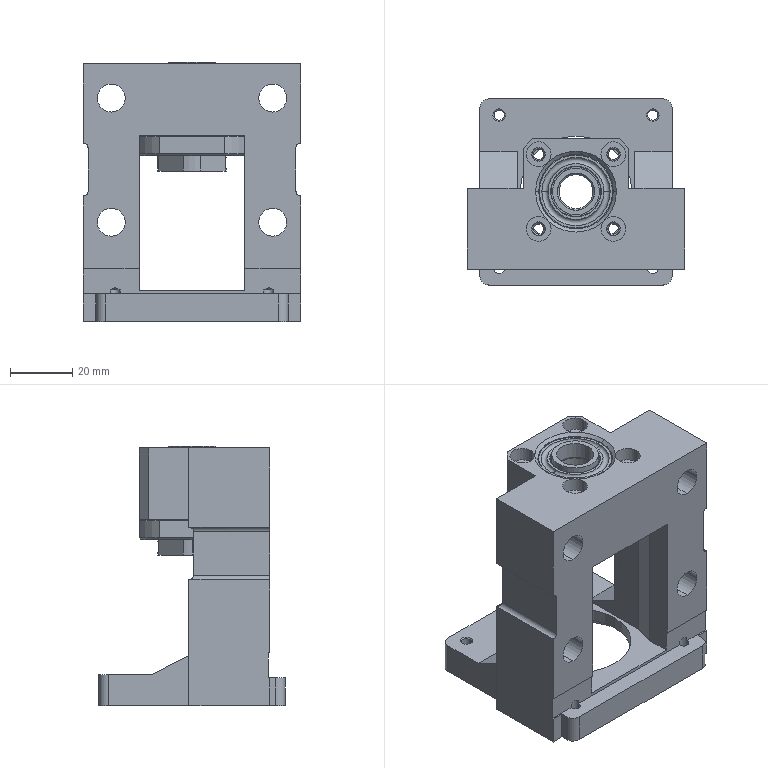Part | STEP file | 001-008-LEF01-d12-F60S-h25 | 9 solids | 355 faces | box 70 x 60 x 83.5 mm | volume 110903 mm3 | cylinder 129 | plane 94 | cone 70 | torus 62 | commonest cylinder face diameters 3.242 x20 3 x8 4.5 x8 8 x8 9 x8 12 x8